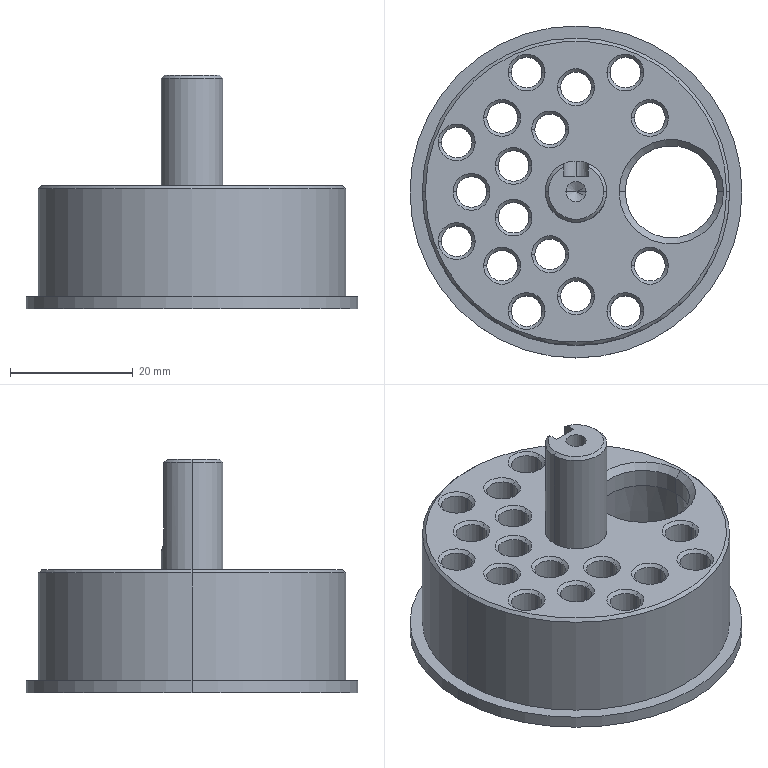Part | SolidWorks | features Chamfer 6, ICE 6, CirPattern 3, HoleWzd 3, Cut 1, Extrusion 1, Fillet 1 | 1 solid | 144 faces | box 54 x 54 x 38 mm | volume 29487 mm3 | cone 85 | cylinder 52 | plane 7 | commonest cylinder face diameters 5 x36 4.2 x4 3.3 x2 4 x2 10 x2 15 x2